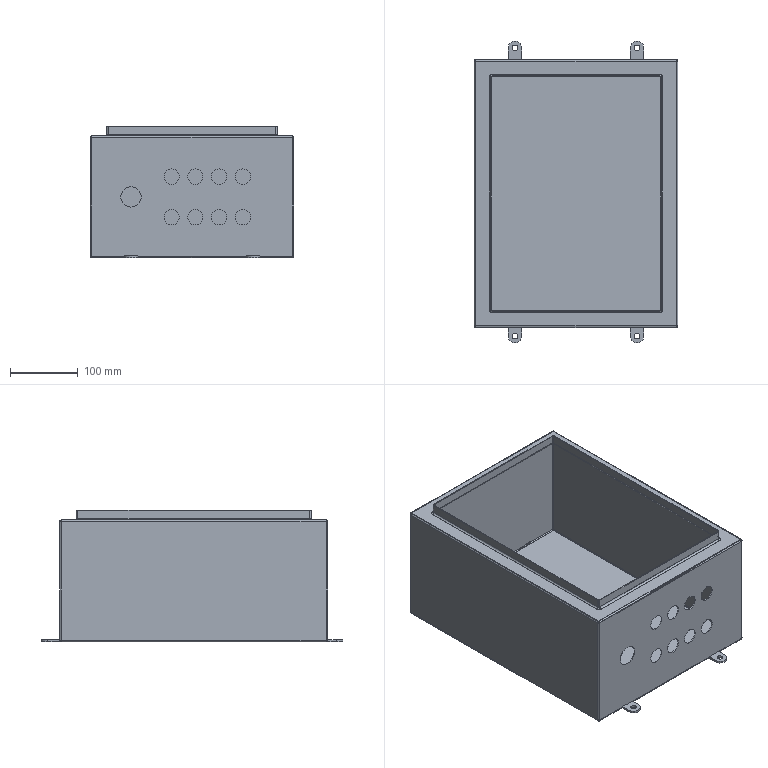Part | SolidWorks | features ICE 3, Fillet 2, Extrusion 1, Shell 1 | 1 solid | 135 faces | box 300 x 445.13 x 194.57 mm | volume 492765 mm3 | cylinder 70 | plane 41 | sphere 16 | torus 8 | commonest cylinder face diameters 4.8 x20 2.4 x16 22.5 x16 8.2 x8 7.2 x4 20 x4